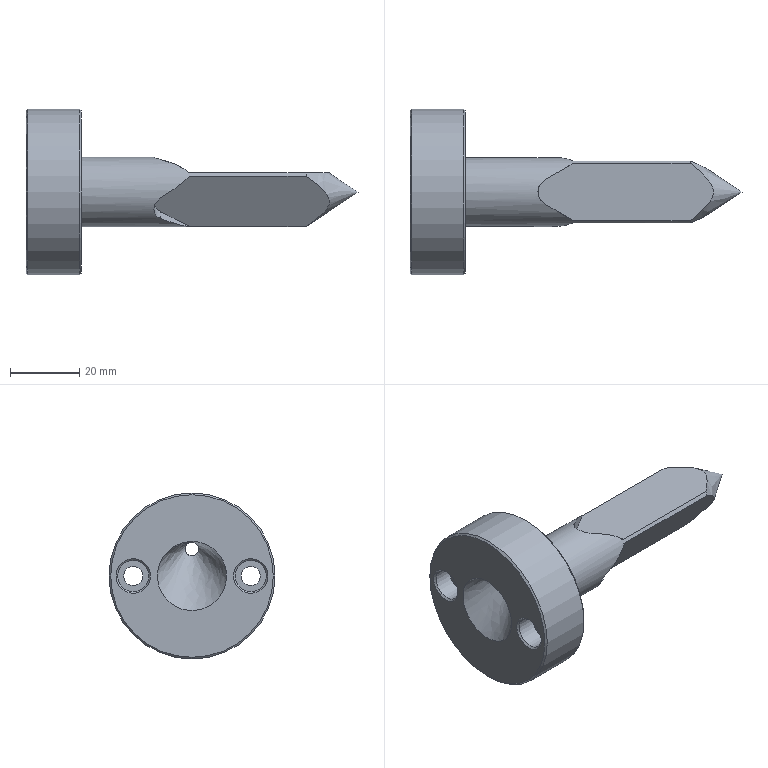NC program | NX | posted with a generic post | part box 96 x 48 x 48 mm
Lines 1763 to 2614 of 9730:
(ZLEVEL_PROFILE_COPY , TOOL : D3R0.5)
N3524 T05 M6
N3526 G54
N3528 G17 G0 G90 X2.228 Y8.23 B0. C0. S6500 M3
N3530 G43 Z30. H5
N3532 Z1.5
N3534 G94 G1 X1.309 Y8.429 Z1.451 F1000.
N3536 X0.209 Y8.524 Z1.393
N3538 X-0.894 Y8.481 Z1.335
N3540 X-1.983 Y8.3 Z1.277
N3542 X-3.041 Y7.983 Z1.219
N3544 X-4.051 Y7.535 Z1.161
N3546 X-4.996 Y6.964 Z1.104
N3548 X-5.862 Y6.279 Z1.046
N3550 X-6.635 Y5.491 Z0.988
N3552 X-6.893 Y5.161 Z0.966
N3554 X-7.147 Y4.833 Z0.944
N3556 X-7.733 Y3.868 Z0.885
N3558 X-8.187 Y2.836 Z0.826
N3560 X-8.503 Y1.753 Z0.767
N3562 X-8.676 Y0.638 Z0.708
N3564 X-8.702 Y-0.49 Z0.648
N3566 X-8.58 Y-1.611 Z0.589
N3568 X-8.314 Y-2.707 Z0.53
N3570 X-7.906 Y-3.759 Z0.471
N3572 X-7.366 Y-4.749 Z0.412
N3574 X-6.701 Y-5.661 Z0.353
N3576 X-5.923 Y-6.477 Z0.294
N3578 X-5.045 Y-7.186 Z0.235
N3580 X-4.082 Y-7.774 Z0.175
N3582 X-3.051 Y-8.231 Z0.116
N3584 X-2.654 Y-8.356 Z0.095
N3586 X-2.258 Y-8.484 Z0.073
N3588 X-1.336 Y-8.681 Z0.023
N3590 X-0.399 Y-8.777 Z-0.026
N3592 X0.018 Z-0.048
N3594 G3 X8.378 Y2.228 R8.678 F2200.
N3596 X5.653 Y6.447 R8.57
N3598 X-6.893 Y5.161 R8.756
N3600 X-2.654 Y-8.356 R8.63
N3602 X0.018 Y-8.777 R8.678
N3604 G1 X0.132 Y-8.765 Z-0.05
N3606 X0.246 Y-8.76 Z-0.052
N3608 X0.36 Y-8.753 Z-0.054
N3610 X0.474 Y-8.746 Z-0.056
N3612 X0.587 Y-8.735 Z-0.058
N3614 X0.701 Y-8.725 Z-0.06
N3616 X0.814 Y-8.712 Z-0.062
N3618 X0.927 Y-8.699 Z-0.064
N3620 X1.04 Y-8.683 Z-0.066
N3622 X1.152 Y-8.665 Z-0.068
N3624 X1.265 Y-8.648 Z-0.07
N3626 X1.377 Y-8.628 Z-0.072
N3628 X1.488 Y-8.607 Z-0.074
N3630 X1.6 Y-8.583 Z-0.076
N3632 X1.711 Y-8.559 Z-0.078
N3634 X1.822 Y-8.534 Z-0.08
N3636 X1.932 Y-8.507 Z-0.082
N3638 X2.042 Y-8.478 Z-0.084
N3640 X2.151 Y-8.448 Z-0.086
N3642 X2.26 Y-8.417 Z-0.088
N3644 X2.369 Y-8.384 Z-0.09
N3646 X2.477 Y-8.351 Z-0.092
N3648 X2.585 Y-8.315 Z-0.094
N3650 X2.694 Y-8.285 Z-0.096
N3652 G3 X8.524 Y1.494 R8.652
N3654 X5.653 Y6.435 R8.537
N3656 X-6.875 Y5.161 R8.724
N3658 X-2.899 Y-8.208 R8.596
N3660 X0.018 Y-8.712 R8.652
N3662 G1 X0.132 Y-8.701 Z-0.098
N3664 X0.246 Y-8.696 Z-0.1
N3666 X0.36 Y-8.689 Z-0.102
N3668 X0.474 Y-8.682 Z-0.104
N3670 X0.587 Y-8.671 Z-0.106
N3672 X0.701 Y-8.661 Z-0.108
N3674 X0.814 Y-8.648 Z-0.11
N3676 X0.927 Y-8.634 Z-0.112
N3678 X1.04 Y-8.618 Z-0.114
N3680 X1.153 Y-8.601 Z-0.116
N3682 X1.265 Y-8.583 Z-0.118
N3684 X1.377 Y-8.563 Z-0.12
N3686 X1.489 Y-8.542 Z-0.122
N3688 X1.6 Y-8.518 Z-0.124
N3690 X1.711 Y-8.494 Z-0.126
N3692 X1.822 Y-8.469 Z-0.128
N3694 X1.932 Y-8.442 Z-0.13
N3696 X2.042 Y-8.413 Z-0.132
N3698 X2.151 Y-8.383 Z-0.134
N3700 X2.261 Y-8.352 Z-0.136
N3702 X2.369 Y-8.319 Z-0.138
N3704 X2.478 Y-8.285 Z-0.14
N3706 X2.585 Y-8.249 Z-0.142
N3708 X2.691 Y-8.209 Z-0.144
N3710 G3 X6.746 Y-5.41 R8.672
N3712 X4.676 Y7.149 R8.531
N3714 G1 X4.432 Y7.297
N3716 X4.33 Y7.361
N3718 X4.187 Y7.439
N3720 G3 X-6.858 Y5.161 R8.697
N3722 X-2.899 Y-8.142 R8.563
N3724 G1 X-2.791 Y-8.178
N3726 G3 X0.018 Y-8.638 R8.672
N3728 G1 X0.132 Y-8.637 Z-0.146
N3730 X0.246 Y-8.632 Z-0.148
N3732 X0.36 Y-8.625 Z-0.15
N3734 X0.474 Y-8.617 Z-0.152
N3736 X0.588 Y-8.607 Z-0.154
N3738 X0.702 Y-8.597 Z-0.156
N3740 X0.815 Y-8.584 Z-0.158
N3742 X0.928 Y-8.57 Z-0.16
N3744 X1.041 Y-8.554 Z-0.162
N3746 X1.154 Y-8.536 Z-0.164
N3748 X1.266 Y-8.519 Z-0.166
N3750 X1.378 Y-8.499 Z-0.168
N3752 X1.49 Y-8.477 Z-0.17
N3754 X1.602 Y-8.453 Z-0.172
N3756 X1.713 Y-8.429 Z-0.174
N3758 X1.824 Y-8.404 Z-0.176
N3760 X1.934 Y-8.377 Z-0.178
N3762 X2.044 Y-8.347 Z-0.18
N3764 X2.154 Y-8.317 Z-0.181
N3766 X2.263 Y-8.286 Z-0.183
N3768 X2.372 Y-8.253 Z-0.185
N3770 X2.48 Y-8.219 Z-0.187
N3772 X2.588 Y-8.182 Z-0.189
N3774 X2.697 Y-8.152 Z-0.191
N3776 G3 X8.568 Y0.761 R8.601
N3778 X3.454 Y7.793 R8.526
N3780 G1 X3.325 Y7.85
N3782 X3.069 Y7.947
N3784 G3 X-3.661 Y7.701 R8.689
N3786 X-8.568 Y0.761 R8.539
N3788 X0.018 Y-8.586 R8.601
N3790 G1 X0.132 Y-8.573 Z-0.193
N3792 X0.246 Y-8.568 Z-0.195
N3794 X0.36 Y-8.561 Z-0.197
N3796 X0.473 Y-8.553 Z-0.199
N3798 X0.587 Y-8.543 Z-0.201
N3800 X0.7 Y-8.533 Z-0.203
N3802 X0.814 Y-8.52 Z-0.205
N3804 X0.927 Y-8.506 Z-0.207
N3806 X1.039 Y-8.489 Z-0.209
N3808 X1.152 Y-8.472 Z-0.211
N3810 X1.264 Y-8.455 Z-0.213
N3812 X1.376 Y-8.434 Z-0.215
N3814 X1.488 Y-8.413 Z-0.217
N3816 X1.599 Y-8.389 Z-0.219
N3818 X1.71 Y-8.365 Z-0.221
N3820 X1.821 Y-8.34 Z-0.223
N3822 X1.931 Y-8.313 Z-0.225
N3824 X2.041 Y-8.283 Z-0.227
N3826 X2.151 Y-8.253 Z-0.229
N3828 X2.26 Y-8.222 Z-0.231
N3830 X2.368 Y-8.189 Z-0.233
N3832 X2.476 Y-8.154 Z-0.235
N3834 X2.584 Y-8.117 Z-0.237
N3836 X2.693 Y-8.088 Z-0.239
N3838 G3 X8.535 Y-0.695 R8.567
N3840 X5.709 Y6.354 R8.421
N3842 X-3.632 Y7.709 R8.644
N3844 X-8.513 Y1.005 R8.508
N3846 X0.017 Y-8.523 R8.567
N3848 G1 X0.131 Y-8.509 Z-0.241
N3850 X0.246 Y-8.504 Z-0.243
N3852 X0.359 Y-8.497 Z-0.245
N3854 X0.473 Y-8.489 Z-0.247
N3856 X0.587 Y-8.479 Z-0.249
N3858 X0.7 Y-8.469 Z-0.251
N3860 X0.813 Y-8.455 Z-0.253
N3862 X0.927 Y-8.442 Z-0.255
N3864 X1.039 Y-8.425 Z-0.257
N3866 X1.152 Y-8.408 Z-0.259
N3868 X1.264 Y-8.39 Z-0.261
N3870 X1.376 Y-8.37 Z-0.263
N3872 X1.488 Y-8.348 Z-0.265
N3874 X1.599 Y-8.324 Z-0.267
N3876 X1.71 Y-8.3 Z-0.269
N3878 X1.821 Y-8.275 Z-0.271
N3880 X1.931 Y-8.248 Z-0.273
N3882 X2.041 Y-8.218 Z-0.275
N3884 X2.15 Y-8.188 Z-0.277
N3886 X2.259 Y-8.157 Z-0.279
N3888 X2.368 Y-8.123 Z-0.281
N3890 X2.476 Y-8.089 Z-0.283
N3892 X2.583 Y-8.052 Z-0.285
N3894 X2.693 Y-8.022 Z-0.287
N3896 G3 X5.025 Y-6.817 R8.526
N3898 X4.187 Y7.419 R8.443
N3900 G1 X4.073 Y7.481
N3902 G3 X-3.679 Y7.682 R8.627
N3904 X-8.412 Y1.494 R8.475
N3906 X0.017 Y-8.46 R8.526
N3908 G1 X0.131 Y-8.445 Z-0.289
N3910 X0.245 Y-8.44 Z-0.291
N3912 X0.359 Y-8.433 Z-0.293
N3914 X0.473 Y-8.425 Z-0.295
N3916 X0.586 Y-8.415 Z-0.297
N3918 X0.7 Y-8.405 Z-0.299
N3920 X0.813 Y-8.391 Z-0.301
N3922 X0.926 Y-8.378 Z-0.303
N3924 X1.039 Y-8.361 Z-0.305
N3926 X1.151 Y-8.343 Z-0.307
N3928 X1.264 Y-8.326 Z-0.309
N3930 X1.376 Y-8.306 Z-0.311
N3932 X1.487 Y-8.284 Z-0.313
N3934 X1.598 Y-8.259 Z-0.315
N3936 X1.709 Y-8.235 Z-0.317
N3938 X1.82 Y-8.21 Z-0.319
N3940 X1.93 Y-8.183 Z-0.321
N3942 X2.04 Y-8.153 Z-0.323
N3944 X2.15 Y-8.123 Z-0.325
N3946 X2.259 Y-8.091 Z-0.327
N3948 X2.367 Y-8.058 Z-0.329
N3950 X2.475 Y-8.023 Z-0.331
N3952 X2.582 Y-7.986 Z-0.333
N3954 X2.693 Y-7.959 Z-0.335
N3956 G3 X8.079 Y2.717 R8.477
N3958 X2.787 Y8.038 R8.456
N3960 G1 X2.721 Y8.06
N3962 G3 X-6.787 Y5.161 R8.552
N3964 X-1.921 Y-8.166 R8.435
N3966 X0.017 Y-8.391 R8.477
N3968 G1 X0.131 Y-8.381 Z-0.337
N3970 X0.246 Y-8.375 Z-0.339
N3972 X0.359 Y-8.369 Z-0.341
N3974 X0.473 Y-8.361 Z-0.343
N3976 X0.587 Y-8.351 Z-0.345
N3978 X0.7 Y-8.34 Z-0.347
N3980 X0.814 Y-8.327 Z-0.349
N3982 X0.927 Y-8.313 Z-0.351
N3984 X1.039 Y-8.296 Z-0.353
N3986 X1.152 Y-8.279 Z-0.355
N3988 X1.264 Y-8.261 Z-0.357
N3990 X1.376 Y-8.241 Z-0.359
N3992 X1.488 Y-8.219 Z-0.361
N3994 X1.599 Y-8.195 Z-0.363
N3996 X1.71 Y-8.17 Z-0.365
N3998 X1.821 Y-8.145 Z-0.367
N4000 X1.931 Y-8.118 Z-0.369
N4002 X2.041 Y-8.088 Z-0.371
N4004 X2.15 Y-8.058 Z-0.373
N4006 X2.259 Y-8.026 Z-0.375
N4008 X2.367 Y-7.993 Z-0.377
N4010 X2.475 Y-7.957 Z-0.379
N4012 X2.582 Y-7.92 Z-0.381
N4014 X2.692 Y-7.89 Z-0.383
N4016 G3 X8.356 Y1.494 R8.46
N4018 X3.454 Y7.773 R8.401
N4020 G1 X3.28 Y7.85
N4022 X3.21 Y7.877
N4024 G3 X-6.576 Y5.406 R8.527
N4026 X-3.143 Y-7.719 R8.395
N4028 X0.017 Y-8.327 R8.46
N4030 G1 X0.131 Y-8.318 Z-0.385
N4032 X0.245 Y-8.311 Z-0.387
N4034 X0.359 Y-8.305 Z-0.389
N4036 X0.473 Y-8.297 Z-0.391
N4038 X0.587 Y-8.287 Z-0.393
N4040 X0.7 Y-8.276 Z-0.395
N4042 X0.814 Y-8.263 Z-0.397
N4044 X0.927 Y-8.249 Z-0.399
N4046 X1.039 Y-8.232 Z-0.401
N4048 X1.152 Y-8.214 Z-0.403
N4050 X1.264 Y-8.197 Z-0.405
N4052 X1.376 Y-8.177 Z-0.407
N4054 X1.488 Y-8.154 Z-0.409
N4056 X1.599 Y-8.13 Z-0.411
N4058 X1.71 Y-8.106 Z-0.413
N4060 X1.821 Y-8.08 Z-0.415
N4062 X1.931 Y-8.053 Z-0.417
N4064 X2.041 Y-8.023 Z-0.419
N4066 X2.15 Y-7.992 Z-0.421
N4068 X2.259 Y-7.961 Z-0.423
N4070 X2.368 Y-7.927 Z-0.425
N4072 X2.475 Y-7.891 Z-0.427
N4074 X2.582 Y-7.854 Z-0.429
N4076 X2.693 Y-7.828 Z-0.431
N4078 G3 X8.172 Y2.228 R8.417
N4080 X2.966 Y7.969 R8.406
N4082 G1 X2.721 Y8.052
N4084 G3 X-6.351 Y5.65 R8.492
N4086 X-2.654 Y-7.83 R8.363
N4088 X0.017 Y-8.265 R8.417
N4090 G1 X0.131 Y-8.254 Z-0.433
N4092 X0.245 Y-8.247 Z-0.435
N4094 X0.359 Y-8.241 Z-0.437
N4096 X0.473 Y-8.233 Z-0.439
N4098 X0.587 Y-8.223 Z-0.441
N4100 X0.7 Y-8.212 Z-0.443
N4102 X0.813 Y-8.199 Z-0.445
N4104 X0.926 Y-8.184 Z-0.447
N4106 X1.152 Y-8.15 Z-0.451
N4108 X1.264 Y-8.132 Z-0.453
N4110 X1.376 Y-8.112 Z-0.455
N4112 X1.487 Y-8.089 Z-0.457
N4114 X1.598 Y-8.065 Z-0.459
N4116 X1.709 Y-8.041 Z-0.461
N4118 X1.82 Y-8.015 Z-0.463
N4120 X1.93 Y-7.988 Z-0.465
N4122 X2.04 Y-7.958 Z-0.467
N4124 X2.149 Y-7.928 Z-0.469
N4126 X2.258 Y-7.895 Z-0.471
N4128 X2.367 Y-7.862 Z-0.473
N4130 X2.474 Y-7.826 Z-0.475
N4132 X2.581 Y-7.789 Z-0.477
N4134 X2.691 Y-7.76 Z-0.479
N4136 G3 X5.574 Y-6.084 R8.397
N4138 X4.676 Y7.092 R8.305
N4140 X-2.41 Y8.148 R8.467
N4142 G1 X-2.592 Y8.095
N4144 G3 X-8.3 Y1.494 R8.362
N4146 X0.017 Y-8.204 R8.397
N4148 G1 X0.131 Y-8.19 Z-0.481
N4150 X0.245 Y-8.183 Z-0.483
N4152 X0.359 Y-8.177 Z-0.485
N4154 X0.473 Y-8.169 Z-0.487
N4156 X0.586 Y-8.159 Z-0.489
N4158 X0.7 Y-8.148 Z-0.491
N4160 X0.813 Y-8.134 Z-0.493
N4162 X0.926 Y-8.12 Z-0.495
N4164 X1.151 Y-8.085 Z-0.499
N4166 X1.263 Y-8.068 Z-0.501
N4168 X1.375 Y-8.048 Z-0.503
N4170 X1.487 Y-8.024 Z-0.505
N4172 X1.598 Y-8. Z-0.507
N4174 X1.709 Y-7.976 Z-0.509
N4176 X1.82 Y-7.951 Z-0.511
N4178 X1.93 Y-7.923 Z-0.513
N4180 X2.039 Y-7.893 Z-0.515
N4182 X2.149 Y-7.863 Z-0.517
N4184 X2.258 Y-7.83 Z-0.519
N4186 X2.366 Y-7.797 Z-0.521
N4188 X2.473 Y-7.76 Z-0.523
N4190 X2.58 Y-7.723 Z-0.525
N4192 X2.69 Y-7.694 Z-0.527
N4194 G3 X6.235 Y-5.35 R8.368
N4196 G1 X6.386 Y-5.181
N4198 G3 X4.629 Y7.117 R8.272
N4200 G1 X4.432 Y7.236
N4202 X4.232 Y7.361
N4204 X3.943 Y7.52
N4206 X3.777 Y7.606
N4208 X3.699 Y7.641
N4210 X3.638 Y7.67
N4212 G3 X-2.368 Y8.157 R8.401
N4214 G1 X-2.582 Y8.095
N4216 G3 X-8.307 Y1.25 R8.325
N4218 X0.017 Y-8.139 R8.368
N4220 G1 X0.131 Y-8.126 Z-0.529
N4222 X0.245 Y-8.119 Z-0.531
N4224 X0.359 Y-8.112 Z-0.533
N4226 X0.473 Y-8.105 Z-0.535
N4228 X0.586 Y-8.095 Z-0.537
N4230 X0.7 Y-8.084 Z-0.539
N4232 X0.813 Y-8.07 Z-0.541
N4234 X0.926 Y-8.055 Z-0.543
N4236 X1.151 Y-8.021 Z-0.547
N4238 X1.263 Y-8.003 Z-0.549
N4240 X1.375 Y-7.983 Z-0.551
N4242 X1.487 Y-7.96 Z-0.553
N4244 X1.598 Y-7.935 Z-0.555
N4246 X1.709 Y-7.911 Z-0.557
N4248 X1.82 Y-7.886 Z-0.559
N4250 X1.93 Y-7.858 Z-0.561
N4252 X2.039 Y-7.828 Z-0.563
N4254 X2.149 Y-7.798 Z-0.565
N4256 X2.257 Y-7.765 Z-0.567
N4258 X2.366 Y-7.731 Z-0.568
N4260 X2.473 Y-7.694 Z-0.57
N4262 X2.58 Y-7.657 Z-0.572
N4264 X2.69 Y-7.627 Z-0.574
N4266 G3 X6.142 Y-5.372 R8.335
N4268 G1 X6.386 Y-5.098
N4270 X6.578 Y-4.862
N4272 G3 X4.616 Y7.117 R8.238
N4274 G1 X4.432 Y7.228
N4276 X4.22 Y7.361
N4278 X3.943 Y7.514
N4280 X3.765 Y7.606
N4282 X3.699 Y7.635
N4284 X3.634 Y7.667
N4286 G3 X-2.361 Y8.156 R8.375
N4288 G1 X-2.571 Y8.095
N4290 G3 X-8.278 Y1.25 R8.291
N4292 X0.017 Y-8.074 R8.335
N4294 G1 X0.131 Y-8.062 Z-0.576
N4296 X0.245 Y-8.055 Z-0.578
N4298 X0.359 Y-8.048 Z-0.58
N4300 X0.473 Y-8.041 Z-0.582
N4302 X0.586 Y-8.031 Z-0.584
N4304 X0.7 Y-8.019 Z-0.586
N4306 X0.813 Y-8.006 Z-0.588
N4308 X0.926 Y-7.991 Z-0.59
N4310 X1.151 Y-7.956 Z-0.594
N4312 X1.263 Y-7.939 Z-0.596
N4314 X1.375 Y-7.918 Z-0.598
N4316 X1.487 Y-7.895 Z-0.6
N4318 X1.598 Y-7.871 Z-0.602
N4320 X1.709 Y-7.847 Z-0.604
N4322 X1.82 Y-7.821 Z-0.606
N4324 X1.93 Y-7.793 Z-0.608
N4326 X2.039 Y-7.763 Z-0.61
N4328 X2.149 Y-7.732 Z-0.612
N4330 X2.257 Y-7.7 Z-0.614
N4332 X2.366 Y-7.665 Z-0.616
N4334 X2.473 Y-7.628 Z-0.618
N4336 X2.58 Y-7.591 Z-0.62
N4338 X2.69 Y-7.562 Z-0.622
N4340 G3 X8.247 Y1.25 R8.303
N4342 X3.454 Y7.748 R8.241
N4344 G1 X3.224 Y7.85
N4346 X2.966 Y7.951
N4348 X2.721 Y8.037
N4350 G3 X-2.41 Y8.139 R8.336
N4352 G1 X-2.56 Y8.095
N4354 G3 X-8.249 Y1.25 R8.254
N4356 X0.017 Y-8.01 R8.303
N4358 G1 X0.131 Y-7.998 Z-0.624
N4360 X0.245 Y-7.991 Z-0.626
N4362 X0.359 Y-7.984 Z-0.628
N4364 X0.472 Y-7.977 Z-0.63
N4366 X0.586 Y-7.967 Z-0.632
N4368 X0.699 Y-7.955 Z-0.634
N4370 X0.813 Y-7.942 Z-0.636
N4372 X0.926 Y-7.927 Z-0.638
N4374 X1.038 Y-7.909 Z-0.64
N4376 X1.151 Y-7.892 Z-0.642
N4378 X1.263 Y-7.875 Z-0.644
N4380 X1.375 Y-7.854 Z-0.646
N4382 X1.486 Y-7.83 Z-0.648
N4384 X1.597 Y-7.806 Z-0.65
N4386 X1.709 Y-7.783 Z-0.652
N4388 X1.819 Y-7.756 Z-0.654
N4390 X1.929 Y-7.728 Z-0.656
N4392 X2.039 Y-7.698 Z-0.658
N4394 X2.148 Y-7.667 Z-0.66
N4396 X2.257 Y-7.634 Z-0.662
N4398 X2.365 Y-7.6 Z-0.664
N4400 X2.472 Y-7.563 Z-0.666
N4402 X2.579 Y-7.525 Z-0.668
N4404 X2.688 Y-7.495 Z-0.67
N4406 G3 X6.142 Y-5.211 R8.271
N4408 G1 X6.236 Y-5.106
N4410 X6.386 Y-4.93
N4412 G3 X4.432 Y7.212 R8.154
N4414 G1 X4.196 Y7.361
N4416 X3.943 Y7.502
N4418 X3.742 Y7.606
N4420 X3.699 Y7.625
N4422 X3.623 Y7.661
N4424 G3 X-2.345 Y8.155 R8.318
N4426 G1 X-2.549 Y8.095
N4428 G3 X-8.244 Y1.005 R8.216
N4430 X0.017 Y-7.944 R8.271
N4432 G1 X0.131 Y-7.934 Z-0.672
N4434 X0.245 Y-7.927 Z-0.674
N4436 X0.359 Y-7.92 Z-0.676
N4438 X0.472 Y-7.913 Z-0.678
N4440 X0.586 Y-7.903 Z-0.68
N4442 X0.7 Y-7.891 Z-0.682
N4444 X0.813 Y-7.877 Z-0.684
N4446 X0.926 Y-7.862 Z-0.686
N4448 X1.038 Y-7.845 Z-0.688
N4450 X1.151 Y-7.828 Z-0.69
N4452 X1.263 Y-7.81 Z-0.692
N4454 X1.375 Y-7.789 Z-0.694
N4456 X1.486 Y-7.765 Z-0.696
N4458 X1.598 Y-7.741 Z-0.698
N4460 X1.709 Y-7.718 Z-0.7
N4462 X1.819 Y-7.691 Z-0.702
N4464 X1.929 Y-7.663 Z-0.704
N4466 X2.039 Y-7.633 Z-0.706
N4468 X2.148 Y-7.602 Z-0.708
N4470 X2.257 Y-7.569 Z-0.71
N4472 X2.365 Y-7.534 Z-0.712
N4474 X2.472 Y-7.497 Z-0.714
N4476 X2.579 Y-7.458 Z-0.716
N4478 X2.688 Y-7.428 Z-0.718
N4480 G3 X8.211 Y1.005 R8.238
N4482 X2.966 Y7.942 R8.169
N4484 G1 X2.721 Y8.029
N4486 G3 X-7.389 Y3.941 R8.271
N4488 X-8.24 Y0.371 R7.96
N4490 X0.016 Y-7.879 R8.238
N4492 G1 X0.13 Y-7.87 Z-0.72
N4494 X0.245 Y-7.863 Z-0.722
N4496 X0.359 Y-7.856 Z-0.724
N4498 X0.472 Y-7.849 Z-0.726
N4500 X0.586 Y-7.839 Z-0.728
N4502 X0.699 Y-7.827 Z-0.73
N4504 X0.813 Y-7.813 Z-0.732
N4506 X0.926 Y-7.798 Z-0.734
N4508 X1.038 Y-7.78 Z-0.736
N4510 X1.151 Y-7.763 Z-0.738
N4512 X1.263 Y-7.746 Z-0.74
N4514 X1.375 Y-7.724 Z-0.742
N4516 X1.486 Y-7.7 Z-0.744
N4518 X1.598 Y-7.676 Z-0.746
N4520 X1.709 Y-7.653 Z-0.748
N4522 X1.819 Y-7.626 Z-0.75
N4524 X1.929 Y-7.598 Z-0.752
N4526 X2.039 Y-7.568 Z-0.754
N4528 X2.148 Y-7.537 Z-0.756
N4530 X2.257 Y-7.504 Z-0.758
N4532 X2.365 Y-7.468 Z-0.76
N4534 X2.472 Y-7.431 Z-0.762
N4536 X2.578 Y-7.392 Z-0.764
N4538 X2.687 Y-7.359 Z-0.766
N4540 G3 X8.206 Y0.516 R8.207
N4542 X3.699 Y7.614 R8.113
N4544 G1 X3.454 Y7.733
N4546 X3.19 Y7.85
N4548 X2.966 Y7.937
N4550 G3 X-6.633 Y5.149 R8.255
N4552 X-8.184 Y-0.231 R8.008
N4554 X0.016 Y-7.812 R8.207
N4556 G1 X0.13 Y-7.805 Z-0.768
N4558 X0.245 Y-7.799 Z-0.77
N4560 X0.359 Y-7.792 Z-0.772
N4562 X0.472 Y-7.785 Z-0.774
N4564 X0.586 Y-7.774 Z-0.776
N4566 X0.7 Y-7.762 Z-0.778
N4568 X0.813 Y-7.749 Z-0.78
N4570 X0.926 Y-7.733 Z-0.782
N4572 X1.038 Y-7.716 Z-0.784
N4574 X1.151 Y-7.699 Z-0.786
N4576 X1.264 Y-7.681 Z-0.788
N4578 X1.375 Y-7.66 Z-0.79
N4580 X1.598 Y-7.611 Z-0.794
N4582 X1.709 Y-7.588 Z-0.796
N4584 X1.82 Y-7.561 Z-0.798
N4586 X1.93 Y-7.533 Z-0.8
N4588 X2.039 Y-7.502 Z-0.802
N4590 X2.149 Y-7.471 Z-0.804
N4592 X2.257 Y-7.438 Z-0.806
N4594 X2.365 Y-7.402 Z-0.808
N4596 X2.472 Y-7.365 Z-0.81
N4598 X2.579 Y-7.325 Z-0.812
N4600 X2.687 Y-7.291 Z-0.814
N4602 G3 X8.05 Y-0.992 R8.174
N4604 X6.083 Y5.798 R8.015
N4606 X-6.218 Y5.65 R8.23
N4608 X-3.387 Y-7.012 R8.096
N4610 G1 X-3.274 Y-7.061
N4612 G3 X0.016 Y-7.745 R8.174
N4614 G1 X0.13 Y-7.741 Z-0.816
N4616 X0.245 Y-7.735 Z-0.818
N4618 X0.359 Y-7.728 Z-0.82
N4620 X0.473 Y-7.721 Z-0.822
N4622 X0.586 Y-7.71 Z-0.824
N4624 X0.7 Y-7.698 Z-0.826
N4626 X0.813 Y-7.685 Z-0.828
N4628 X0.926 Y-7.668 Z-0.83
N4630 X1.039 Y-7.651 Z-0.832
N4632 X1.151 Y-7.635 Z-0.834
N4634 X1.264 Y-7.617 Z-0.836
N4636 X1.376 Y-7.595 Z-0.838
N4638 X1.598 Y-7.546 Z-0.842
N4640 X1.71 Y-7.523 Z-0.844
N4642 X1.82 Y-7.496 Z-0.846
N4644 X1.93 Y-7.468 Z-0.848
N4646 X2.04 Y-7.437 Z-0.85
N4648 X2.149 Y-7.406 Z-0.852
N4650 X2.258 Y-7.372 Z-0.854
N4652 X2.365 Y-7.336 Z-0.856
N4654 X2.473 Y-7.299 Z-0.858
N4656 X2.579 Y-7.259 Z-0.86
N4658 X2.686 Y-7.223 Z-0.862
N4660 G3 X5.75 Y-5.303 R8.151
N4662 G1 X5.778 Y-5.275
N4664 G3 X4.38 Y7.214 R8.03
N4666 G1 X4.187 Y7.335
N4668 G3 X-6.403 Y5.406 R8.203
N4670 X-3.387 Y-6.944 R8.063
N4672 G1 X-3.281 Y-6.991
N4674 G3 X0.016 Y-7.679 R8.151
N4676 G1 X0.13 Y-7.677 Z-0.864
N4678 X0.244 Y-7.671 Z-0.866
N4680 X0.358 Y-7.664 Z-0.868
N4682 X0.472 Y-7.657 Z-0.87
N4684 X0.586 Y-7.646 Z-0.872
N4686 X0.7 Y-7.634 Z-0.874
N4688 X0.813 Y-7.62 Z-0.876
N4690 X0.926 Y-7.604 Z-0.878
N4692 X1.039 Y-7.587 Z-0.88
N4694 X1.152 Y-7.57 Z-0.882
N4696 X1.264 Y-7.552 Z-0.884
N4698 X1.376 Y-7.53 Z-0.886
N4700 X1.487 Y-7.506 Z-0.888
N4702 X1.598 Y-7.481 Z-0.89
N4704 X1.71 Y-7.459 Z-0.892
N4706 X1.82 Y-7.431 Z-0.894
N4708 X1.93 Y-7.403 Z-0.896
N4710 X2.04 Y-7.372 Z-0.898
N4712 X2.149 Y-7.341 Z-0.9
N4714 X2.258 Y-7.307 Z-0.902
N4716 X2.365 Y-7.27 Z-0.904
N4718 X2.473 Y-7.233 Z-0.906
N4720 X2.579 Y-7.192 Z-0.908
N4722 X2.688 Y-7.161 Z-0.91
N4724 G3 X8.089 Y1.005 R8.105
N4726 X5.409 Y6.434 R7.989
N4728 X-6.185 Y5.65 R8.168
N4730 X-3.387 Y-6.877 R8.029
N4732 G1 X-3.143 Y-6.985
N4734 G3 X0.016 Y-7.619 R8.105
N4736 G1 X0.13 Y-7.613 Z-0.912
N4738 X0.244 Y-7.606 Z-0.914
N4740 X0.358 Y-7.6 Z-0.916
N4742 X0.472 Y-7.592 Z-0.918
N4744 X0.586 Y-7.582 Z-0.92
N4746 X0.699 Y-7.57 Z-0.922
N4748 X0.813 Y-7.556 Z-0.924
N4750 X0.925 Y-7.54 Z-0.926
N4752 X1.038 Y-7.522 Z-0.928
N4754 X1.151 Y-7.506 Z-0.93
N4756 X1.263 Y-7.488 Z-0.932
N4758 X1.375 Y-7.465 Z-0.934
N4760 X1.486 Y-7.441 Z-0.936
N4762 X1.597 Y-7.417 Z-0.938
N4764 X1.709 Y-7.394 Z-0.94
N4766 X1.819 Y-7.366 Z-0.942
N4768 X1.929 Y-7.338 Z-0.944
N4770 X2.039 Y-7.307 Z-0.946
N4772 X2.148 Y-7.276 Z-0.948
N4774 X2.256 Y-7.242 Z-0.95
N4776 X2.364 Y-7.205 Z-0.952
N4778 X2.471 Y-7.167 Z-0.954
N4780 X2.577 Y-7.126 Z-0.956
N4782 X2.685 Y-7.091 Z-0.958
N4784 G3 X7.119 Y-3.299 R8.092
N4786 X4.432 Y7.166 R7.957
N4788 G1 X4.309 Y7.243
N4790 G3 X-6.369 Y5.406 R8.128
N4792 X-2.899 Y-7.017 R8.002
N4794 G1 X-2.654 Y-7.104
N4796 G3 X0.016 Y-7.551 R8.092
N4798 G1 X0.13 Y-7.549 Z-0.96
N4800 X0.244 Y-7.542 Z-0.962
N4802 X0.358 Y-7.536 Z-0.964
N4804 X0.472 Y-7.528 Z-0.966
N4806 X0.586 Y-7.518 Z-0.968
N4808 X0.7 Y-7.506 Z-0.97
N4810 X0.813 Y-7.492 Z-0.972
N4812 X0.926 Y-7.475 Z-0.974
N4814 X1.038 Y-7.458 Z-0.976
N4816 X1.151 Y-7.442 Z-0.978
N4818 X1.264 Y-7.423 Z-0.98
N4820 X1.375 Y-7.4 Z-0.982
N4822 X1.487 Y-7.376 Z-0.984
N4824 X1.598 Y-7.352 Z-0.986
N4826 X1.709 Y-7.329 Z-0.988
N4828 X1.82 Y-7.301 Z-0.99
N4830 X1.93 Y-7.273 Z-0.992
N4832 X2.04 Y-7.242 Z-0.994
N4834 X2.149 Y-7.21 Z-0.996
N4836 X2.257 Y-7.176 Z-0.998
N4838 X2.364 Y-7.139 Z-1.
N4840 X2.471 Y-7.1 Z-1.002
N4842 X2.577 Y-7.059 Z-1.004
N4844 X2.685 Y-7.023 Z-1.006
N4846 G3 X2.966 Y-6.916 R7.999
N4848 X7.377 Y3.694 R7.981
N4850 X1.744 Y8.285 R8.013
N4852 X-7.142 Y4.183 R8.065
N4854 X-0.944 Y-7.433 R7.989
N4856 X0.016 Y-7.489 R7.999
N4858 G1 X0.13 Y-7.485 Z-1.008
N4860 X0.244 Y-7.478 Z-1.01
N4862 X0.358 Y-7.472 Z-1.012
N4864 X0.472 Y-7.464 Z-1.013
N4866 X0.586 Y-7.454 Z-1.015
N4868 X0.699 Y-7.441 Z-1.017
N4870 X0.812 Y-7.428 Z-1.019
N4872 X0.925 Y-7.411 Z-1.021
N4874 X1.038 Y-7.393 Z-1.023
N4876 X1.151 Y-7.378 Z-1.025
N4878 X1.263 Y-7.359 Z-1.027
N4880 X1.375 Y-7.335 Z-1.029
N4882 X1.486 Y-7.311 Z-1.031
N4884 X1.598 Y-7.288 Z-1.033
N4886 X1.709 Y-7.264 Z-1.035
N4888 X1.819 Y-7.236 Z-1.037
N4890 X1.929 Y-7.208 Z-1.039
N4892 X2.039 Y-7.177 Z-1.041
N4894 X2.148 Y-7.145 Z-1.043
N4896 X2.256 Y-7.11 Z-1.045
N4898 X2.364 Y-7.073 Z-1.047
N4900 X2.47 Y-7.034 Z-1.049
N4902 X2.576 Y-6.993 Z-1.051
N4904 X2.684 Y-6.956 Z-1.053
N4906 G3 X2.966 Y-6.849 R7.949
N4908 X7.354 Y3.694 R7.947
N4910 X1.744 Y8.282 R7.978
N4912 X-7.121 Y4.183 R8.031
N4914 X-0.944 Y-7.369 R7.957
N4916 X0.015 Y-7.425 R7.949
N4918 G1 X0.13 Y-7.421 Z-1.055
N4920 X0.244 Y-7.414 Z-1.057
N4922 X0.358 Y-7.407 Z-1.059
N4924 X0.472 Y-7.4 Z-1.061
N4926 X0.586 Y-7.39 Z-1.063
N4928 X0.699 Y-7.377 Z-1.065
N4930 X0.812 Y-7.363 Z-1.067
N4932 X0.925 Y-7.346 Z-1.069
N4934 X1.038 Y-7.329 Z-1.071
N4936 X1.151 Y-7.314 Z-1.073
N4938 X1.263 Y-7.294 Z-1.075
N4940 X1.375 Y-7.271 Z-1.077
N4942 X1.486 Y-7.246 Z-1.079
N4944 X1.597 Y-7.223 Z-1.081
N4946 X1.709 Y-7.199 Z-1.083
N4948 X1.819 Y-7.171 Z-1.085
N4950 X1.929 Y-7.143 Z-1.087
N4952 X2.039 Y-7.112 Z-1.089
N4954 X2.148 Y-7.079 Z-1.091
N4956 X2.256 Y-7.044 Z-1.093
N4958 X2.363 Y-7.007 Z-1.095
N4960 X2.47 Y-6.967 Z-1.097
N4962 X2.576 Y-6.927 Z-1.099
N4964 X2.684 Y-6.893 Z-1.101
N4966 G3 X7.644 Y-1.684 R7.99
N4968 G1 X7.714 Y-1.439
N4970 X7.772 Y-1.195
N4972 X7.827 Y-0.95
N4974 X7.852 Y-0.798
N4976 X7.906 Y-0.461
N4978 X7.932 Y-0.217
N4980 X7.956 Y0.028
N4982 X7.97 Y0.272
N4984 G3 X3.108 Y7.85 R7.896
N4986 G1 X2.966 Y7.905
N4988 G3 X-6.824 Y4.672 R8.014
N4990 X-2.167 Y-7.062 R7.913
N4992 G1 X-1.921 Y-7.126
N4994 G3 X0.015 Y-7.359 R7.99
N4996 G1 X0.129 Y-7.357 Z-1.103
N4998 X0.244 Y-7.35 Z-1.105
N5000 X0.358 Y-7.343 Z-1.107
N5002 X0.472 Y-7.336 Z-1.109
N5004 X0.586 Y-7.326 Z-1.111
N5006 X0.699 Y-7.313 Z-1.113
N5008 X0.812 Y-7.299 Z-1.115
N5010 X0.925 Y-7.282 Z-1.117
N5012 X1.038 Y-7.264 Z-1.119
N5014 X1.151 Y-7.25 Z-1.121
N5016 X1.263 Y-7.229 Z-1.123
N5018 X1.375 Y-7.206 Z-1.125
N5020 X1.486 Y-7.181 Z-1.127
N5022 X1.598 Y-7.159 Z-1.129
N5024 X1.709 Y-7.134 Z-1.131
N5026 X1.819 Y-7.106 Z-1.133
N5028 X1.929 Y-7.077 Z-1.135
N5030 X2.039 Y-7.047 Z-1.137
N5032 X2.147 Y-7.014 Z-1.139
N5034 X2.256 Y-6.978 Z-1.141
N5036 X2.363 Y-6.941 Z-1.143
N5038 X2.469 Y-6.901 Z-1.145
N5040 X2.575 Y-6.861 Z-1.147
N5042 X2.684 Y-6.828 Z-1.149
N5044 G3 X7.87 Y-0.461 R7.951
N5046 X3.625 Y7.606 R7.844
N5048 G1 X3.454 Y7.689
N5050 G3 X-6.299 Y5.406 R8.002
N5052 X-2.899 Y-6.751 R7.87
N5054 G1 X-2.654 Y-6.84
N5056 G3 X0.015 Y-7.296 R7.951
N5058 G1 X0.129 Y-7.293 Z-1.151
N5060 X0.244 Y-7.286 Z-1.153
N5062 X0.358 Y-7.279 Z-1.155
N5064 X0.472 Y-7.272 Z-1.157
N5066 X0.585 Y-7.262 Z-1.159
N5068 X0.699 Y-7.249 Z-1.161
N5070 X0.812 Y-7.234 Z-1.163
N5072 X0.925 Y-7.217 Z-1.165
N5074 X1.038 Y-7.2 Z-1.167
N5076 X1.151 Y-7.185 Z-1.169
N5078 X1.263 Y-7.165 Z-1.171
N5080 X1.374 Y-7.141 Z-1.173
N5082 X1.486 Y-7.117 Z-1.175
N5084 X1.597 Y-7.095 Z-1.177
N5086 X1.708 Y-7.069 Z-1.179
N5088 X1.819 Y-7.041 Z-1.181
N5090 X1.929 Y-7.012 Z-1.183
N5092 X2.038 Y-6.982 Z-1.185
N5094 X2.147 Y-6.949 Z-1.187
N5096 X2.255 Y-6.913 Z-1.189
N5098 X2.362 Y-6.875 Z-1.191
N5100 X2.468 Y-6.835 Z-1.193
N5102 X2.575 Y-6.795 Z-1.195
N5104 X2.685 Y-6.766 Z-1.197
N5106 G3 X7.825 Y-0.465 R7.903
N5108 X5.501 Y6.267 R7.766
N5110 X-6.085 Y5.65 R7.97
N5112 X-2.899 Y-6.684 R7.835
N5114 G1 X-2.654 Y-6.774
N5116 G3 X0.015 Y-7.235 R7.903
N5118 G1 X0.129 Y-7.229 Z-1.199
N5120 X0.243 Y-7.222 Z-1.201
N5122 X0.357 Y-7.215 Z-1.203
N5124 X0.471 Y-7.208 Z-1.205
N5126 X0.585 Y-7.198 Z-1.207
N5128 X0.698 Y-7.184 Z-1.209
N5130 X0.812 Y-7.17 Z-1.211
N5132 X0.924 Y-7.153 Z-1.213
N5134 X1.037 Y-7.135 Z-1.215
N5136 X1.15 Y-7.121 Z-1.217
N5138 X1.262 Y-7.1 Z-1.219
N5140 X1.374 Y-7.076 Z-1.221
N5142 X1.485 Y-7.052 Z-1.223
N5144 X1.597 Y-7.031 Z-1.225
N5146 X1.707 Y-7.005 Z-1.227
N5148 X1.818 Y-6.977 Z-1.229
N5150 X1.927 Y-6.948 Z-1.231
N5152 X2.037 Y-6.917 Z-1.233
N5154 X2.146 Y-6.884 Z-1.235
N5156 X2.253 Y-6.847 Z-1.237
N5158 X2.36 Y-6.809 Z-1.239
N5160 X2.466 Y-6.769 Z-1.241
N5162 X2.573 Y-6.731 Z-1.243
N5164 X2.681 Y-6.696 Z-1.245
N5166 G3 X7.704 Y-0.95 R7.888
N5168 X3.601 Y7.606 R7.774
N5170 G1 X3.454 Y7.677
N5172 G3 X-6.264 Y5.406 R7.933
N5174 X-3.143 Y-6.517 R7.802
N5176 G1 X-2.899 Y-6.617
N5178 G3 X0.015 Y-7.167 R7.888
N5180 G1 X0.129 Y-7.165 Z-1.247
N5182 X0.243 Y-7.158 Z-1.249
N5184 X0.357 Y-7.151 Z-1.251
N5186 X0.471 Y-7.144 Z-1.253
N5188 X0.585 Y-7.134 Z-1.255
N5190 X0.699 Y-7.12 Z-1.257
N5192 X0.812 Y-7.105 Z-1.259
N5194 X0.925 Y-7.088 Z-1.261
N5196 X1.037 Y-7.071 Z-1.263
N5198 X1.15 Y-7.056 Z-1.265
N5200 X1.263 Y-7.035 Z-1.267
N5202 X1.374 Y-7.011 Z-1.269
N5204 X1.485 Y-6.987 Z-1.271
N5206 X1.597 Y-6.966 Z-1.273
N5208 X1.708 Y-6.939 Z-1.275
N5210 X1.818 Y-6.912 Z-1.277
N5212 X1.928 Y-6.882 Z-1.279
N5214 X2.038 Y-6.851 Z-1.281
N5216 X2.146 Y-6.818 Z-1.283
N5218 X2.254 Y-6.781 Z-1.285
N5220 X2.361 Y-6.742 Z-1.287